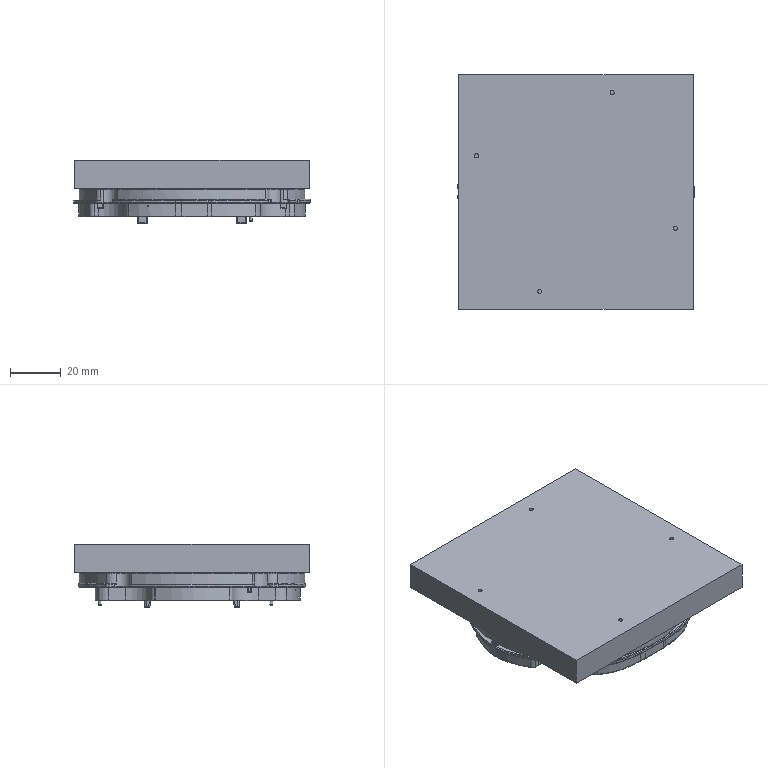NC program | NX | posted with a generic post | part box 92.935 x 92.1 x 24.829 mm
Lines 2470 to 3402 of 7643:
(PLANAR_MILL , TOOL : D3-9-D4-50-3T-ROUGH)
N4914 T15 M6
N4916 G53
N4918 G17 G0 G90 X17.469 Y27.537 S3500 M3
N4920 G43 Z21. H15
N4922 Z1.
N4924 G94 G1 Y26.515 Z0.991 F800.
N4926 X23.689 Z0.937
N4928 Y33.012 Z0.88
N4930 X17.801 Z0.829
N4932 X17.469 Z0.826
N4934 Y26.515 Z0.769
N4936 X23.689 Z0.715
N4938 Y33.012 Z0.658
N4940 X17.801 Z0.607
N4942 X17.469 Z0.604
N4944 Y26.515 Z0.547
N4946 X23.689 Z0.493
N4948 Y33.012 Z0.436
N4950 X17.801 Z0.385
N4952 X17.469 Z0.382
N4954 Y26.515 Z0.325
N4956 X23.689 Z0.271
N4958 Y33.012 Z0.214
N4960 X17.801 Z0.163
N4962 X17.469 Z0.16
N4964 Y26.515 Z0.103
N4966 X23.689 Z0.049
N4968 Y33.012 Z-0.008
N4970 X17.801 Z-0.059
N4972 X17.469 Z-0.062
N4974 Y26.515 Z-0.119
N4976 X23.689 Z-0.173
N4978 Y33.012 Z-0.23
N4980 X17.801 Z-0.281
N4982 X17.469 Z-0.284
N4984 Y26.515 Z-0.341
N4986 X23.689 Z-0.395
N4988 Y33.012 Z-0.452
N4990 X17.801 Z-0.503
N4992 X17.469 Z-0.506
N4994 Y26.515 Z-0.563
N4996 X23.689 Z-0.617
N4998 Y33.012 Z-0.674
N5000 X17.801 Z-0.725
N5002 X17.469 Z-0.728
N5004 Y26.515 Z-0.785
N5006 X23.689 Z-0.839
N5008 Y33.012 Z-0.896
N5010 X17.801 Z-0.947
N5012 X17.469 Z-0.95
N5014 Y26.515 Z-1.007
N5016 X23.689 Z-1.061
N5018 Y33.012 Z-1.118
N5020 X17.801 Z-1.169
N5022 X17.469 Z-1.172
N5024 Y26.515 Z-1.229
N5026 X23.689 Z-1.283
N5028 Y33.012 Z-1.34
N5030 X17.801 Z-1.391
N5032 X17.469 Z-1.394
N5034 Y26.515 Z-1.451
N5036 X23.689 Z-1.505
N5038 Y33.012 Z-1.562
N5040 X17.801 Z-1.613
N5042 X17.469 Z-1.616
N5044 Y26.515 Z-1.673
N5046 X23.689 Z-1.727
N5048 Y33.012 Z-1.784
N5050 X17.801 Z-1.835
N5052 X17.469 Z-1.838
N5054 Y26.515 Z-1.895
N5056 X23.689 Z-1.949
N5058 Y33.012 Z-2.006
N5060 X17.801 Z-2.057
N5062 X17.469 Z-2.06
N5064 Y26.515 Z-2.116
N5066 X23.689 Z-2.171
N5068 Y33.012 Z-2.227
N5070 X17.801 Z-2.279
N5072 X17.469 Z-2.282
N5074 Y26.515 Z-2.338
N5076 X23.689 Z-2.393
N5078 Y33.012 Z-2.449
N5080 X17.801 Z-2.501
N5082 X17.469 Z-2.504
N5084 Y26.515 Z-2.56
N5086 X23.689 Z-2.615
N5088 Y33.012 Z-2.671
N5090 X17.801 Z-2.723
N5092 X17.469 Z-2.726
N5094 Y26.515 Z-2.782
N5096 X23.689 Z-2.837
N5098 Y33.012 Z-2.893
N5100 X17.801 Z-2.945
N5102 X17.469 Z-2.948
N5104 Y26.515 Z-3.004
N5106 X23.689 Z-3.059
N5108 Y33.012 Z-3.115
N5110 X17.801 Z-3.167
N5112 X17.469 Z-3.17
N5114 Y26.515 Z-3.226
N5116 X23.689 Z-3.281
N5118 Y33.012 Z-3.337
N5120 X17.801 Z-3.389
N5122 X17.469 Z-3.392
N5124 Y26.515 Z-3.448
N5126 X23.689 Z-3.503
N5128 Y33.012 Z-3.559
N5130 X17.801 Z-3.611
N5132 X17.469 Z-3.614
N5134 Y26.515 Z-3.67
N5136 X23.689 Z-3.725
N5138 Y33.012 Z-3.781
N5140 X17.801 Z-3.833
N5142 X17.469 Z-3.836
N5144 Y26.515 Z-3.892
N5146 X23.689 Z-3.947
N5148 Y33.012 Z-4.003
N5150 X17.801 Z-4.055
N5152 X17.469 Z-4.058
N5154 Y26.515 Z-4.114
N5156 X23.689 Z-4.169
N5158 Y33.012 Z-4.225
N5160 X17.801 Z-4.277
N5162 X17.469 Z-4.279
N5164 Y26.515 Z-4.336
N5166 X23.689 Z-4.39
N5168 Y33.012 Z-4.447
N5170 X17.801 Z-4.499
N5172 X17.469 Z-4.501
N5174 Y26.515 Z-4.558
N5176 X23.689 Z-4.612
N5178 Y33.012 Z-4.669
N5180 X17.801 Z-4.721
N5182 X17.469 Z-4.723
N5184 Y26.515 Z-4.78
N5186 X23.689 Z-4.834
N5188 Y33.012 Z-4.891
N5190 X17.801 Z-4.942
N5192 X17.469 Z-4.945
N5194 Y26.515 Z-5.002
N5196 X23.689 Z-5.056
N5198 Y33.012 Z-5.113
N5200 X17.801 Z-5.164
N5202 X17.469 Z-5.167
N5204 Y26.515 Z-5.224
N5206 X23.689 Z-5.278
N5208 Y33.012 Z-5.335
N5210 X17.801 Z-5.386
N5212 X17.469 Z-5.389
N5214 Y26.515 Z-5.446
N5216 X23.689 Z-5.5
N5218 Y33.012 Z-5.557
N5220 X17.801 Z-5.608
N5222 X17.469 Z-5.611
N5224 Y26.515 Z-5.668
N5226 X23.689 Z-5.722
N5228 Y33.012 Z-5.779
N5230 X17.801 Z-5.83
N5232 X17.469 Z-5.833
N5234 Y26.515 Z-5.89
N5236 X23.689 Z-5.944
N5238 Y33.012 Z-6.001
N5240 X17.801 Z-6.052
N5242 X17.469 Z-6.055
N5244 Y26.515 Z-6.112
N5246 X23.689 Z-6.166
N5248 Y33.012 Z-6.223
N5250 X17.801 Z-6.274
N5252 X17.469 Z-6.277
N5254 Y26.515 Z-6.334
N5256 X23.689 Z-6.388
N5258 Y33.012 Z-6.445
N5260 X17.801 Z-6.496
N5262 X17.469 Z-6.499
N5264 Y26.515 Z-6.556
N5266 X23.689 Z-6.61
N5268 Y33.012 Z-6.667
N5270 X17.801 Z-6.718
N5272 X17.469 Z-6.721
N5274 Y26.515 Z-6.778
N5276 X23.689 Z-6.832
N5278 Y33.012 Z-6.889
N5280 X17.801 Z-6.94
N5282 X17.469 Z-6.943
N5284 Y26.515 Z-7.
N5286 X23.689 Z-7.054
N5288 Y33.012 Z-7.111
N5290 X17.801 Z-7.162
N5292 X17.469 Z-7.165
N5294 Y26.515 Z-7.222
N5296 X23.689 Z-7.276
N5298 Y33.012 Z-7.333
N5300 X17.801 Z-7.384
N5302 X17.469 Z-7.387
N5304 Y26.515 Z-7.444
N5306 X23.689 Z-7.498
N5308 Y33.012 Z-7.555
N5310 X17.801 Z-7.606
N5312 X17.469 Z-7.609
N5314 Y26.515 Z-7.666
N5316 X23.689 Z-7.72
N5318 Y33.012 Z-7.777
N5320 X17.801 Z-7.828
N5322 X17.469 Z-7.831
N5324 Y26.515 Z-7.888
N5326 X23.689 Z-7.942
N5328 Y33.012 Z-7.999
N5330 X17.801 Z-8.05
N5332 X17.469 Z-8.053
N5334 Y26.515 Z-8.11
N5336 X23.689 Z-8.164
N5338 Y33.012 Z-8.221
N5340 X17.801 Z-8.272
N5342 X17.469 Z-8.275
N5344 Y29.763 Z-8.303
N5346 Y26.515
N5348 X23.689
N5350 Y33.012
N5352 X17.801
N5354 X17.469
N5356 Y29.763
N5358 Z-7.303
N5360 G0 Z21.
N5362 X32.982 Y3.515
N5364 Z1.
N5366 G1 X37.639 Z0.959
N5368 X37.963 Y3.839 Z0.955
N5370 X37.928 Y10.192 Z0.9
N5372 X37.646 Y10.474 Z0.896
N5374 X37.558 Y10.509
N5376 X37.463 Z0.895
N5378 X32.293 Z0.85
N5380 X31.969 Y10.185 Z0.846
N5382 Y3.839 Z0.79
N5384 X32.293 Y3.515 Z0.786
N5386 X37.639 Z0.74
N5388 X37.963 Y3.839 Z0.736
N5390 X37.928 Y10.192 Z0.68
N5392 X37.646 Y10.474 Z0.677
N5394 X37.558 Y10.509 Z0.676
N5396 X37.463 Z0.675
N5398 X32.293 Z0.63
N5400 X31.969 Y10.185 Z0.626
N5402 Y3.839 Z0.57
N5404 X32.293 Y3.515 Z0.566
N5406 X37.639 Z0.52
N5408 X37.963 Y3.839 Z0.516
N5410 X37.928 Y10.192 Z0.46
N5412 X37.646 Y10.474 Z0.457
N5414 X37.558 Y10.509 Z0.456
N5416 X37.463 Z0.455
N5418 X32.293 Z0.41
N5420 X31.969 Y10.185 Z0.406
N5422 Y3.839 Z0.351
N5424 X32.293 Y3.515 Z0.347
N5426 X37.639 Z0.3
N5428 X37.963 Y3.839 Z0.296
N5430 X37.928 Y10.192 Z0.241
N5432 X37.646 Y10.474 Z0.237
N5434 X37.558 Y10.509 Z0.236
N5436 X37.463 Z0.235
N5438 X32.293 Z0.19
N5440 X31.969 Y10.185 Z0.186
N5442 Y3.839 Z0.131
N5444 X32.293 Y3.515 Z0.127
N5446 X37.639 Z0.08
N5448 X37.963 Y3.839 Z0.076
N5450 X37.928 Y10.192 Z0.021
N5452 X37.646 Y10.474 Z0.017
N5454 X37.558 Y10.509 Z0.016
N5456 X37.463
N5458 X32.293 Z-0.03
N5460 X31.969 Y10.185 Z-0.034
N5462 Y3.839 Z-0.089
N5464 X32.293 Y3.515 Z-0.093
N5466 X37.639 Z-0.14
N5468 X37.963 Y3.839 Z-0.144
N5470 X37.928 Y10.192 Z-0.199
N5472 X37.646 Y10.474 Z-0.203
N5474 X37.558 Y10.509
N5476 X37.463 Z-0.204
N5478 X32.293 Z-0.249
N5480 X31.969 Y10.185 Z-0.253
N5482 Y3.839 Z-0.309
N5484 X32.293 Y3.515 Z-0.313
N5486 X37.639 Z-0.359
N5488 X37.963 Y3.839 Z-0.363
N5490 X37.928 Y10.192 Z-0.419
N5492 X37.646 Y10.474 Z-0.422
N5494 X37.558 Y10.509 Z-0.423
N5496 X37.463 Z-0.424
N5498 X32.293 Z-0.469
N5500 X31.969 Y10.185 Z-0.473
N5502 Y3.839 Z-0.528
N5504 X32.293 Y3.515 Z-0.532
N5506 X37.639 Z-0.579
N5508 X37.963 Y3.839 Z-0.583
N5510 X37.928 Y10.192 Z-0.639
N5512 X37.646 Y10.474 Z-0.642
N5514 X37.558 Y10.509 Z-0.643
N5516 X37.463 Z-0.644
N5518 X32.293 Z-0.689
N5520 X31.969 Y10.185 Z-0.693
N5522 Y3.839 Z-0.748
N5524 X32.293 Y3.515 Z-0.752
N5526 X37.639 Z-0.799
N5528 X37.963 Y3.839 Z-0.803
N5530 X37.928 Y10.192 Z-0.858
N5532 X37.646 Y10.474 Z-0.862
N5534 X37.558 Y10.509 Z-0.863
N5536 X37.463 Z-0.864
N5538 X32.293 Z-0.909
N5540 X31.969 Y10.185 Z-0.913
N5542 Y3.839 Z-0.968
N5544 X32.293 Y3.515 Z-0.972
N5546 X37.639 Z-1.019
N5548 X37.963 Y3.839 Z-1.023
N5550 X37.928 Y10.192 Z-1.078
N5552 X37.646 Y10.474 Z-1.082
N5554 X37.558 Y10.509 Z-1.083
N5556 X37.463
N5558 X32.293 Z-1.128
N5560 X31.969 Y10.185 Z-1.132
N5562 Y3.839 Z-1.188
N5564 X32.293 Y3.515 Z-1.192
N5566 X37.639 Z-1.238
N5568 X37.963 Y3.839 Z-1.242
N5570 X37.928 Y10.192 Z-1.298
N5572 X37.646 Y10.474 Z-1.301
N5574 X37.558 Y10.509 Z-1.302
N5576 X37.463 Z-1.303
N5578 X32.293 Z-1.348
N5580 X31.969 Y10.185 Z-1.352
N5582 Y3.839 Z-1.408
N5584 X32.293 Y3.515 Z-1.412
N5586 X37.639 Z-1.458
N5588 X37.963 Y3.839 Z-1.462
N5590 X37.928 Y10.192 Z-1.518
N5592 X37.646 Y10.474 Z-1.521
N5594 X37.558 Y10.509 Z-1.522
N5596 X37.463 Z-1.523
N5598 X32.293 Z-1.568
N5600 X31.969 Y10.185 Z-1.572
N5602 Y3.839 Z-1.627
N5604 X32.293 Y3.515 Z-1.631
N5606 X37.639 Z-1.678
N5608 X37.963 Y3.839 Z-1.682
N5610 X37.928 Y10.192 Z-1.738
N5612 X37.646 Y10.474 Z-1.741
N5614 X37.558 Y10.509 Z-1.742
N5616 X37.463 Z-1.743
N5618 X32.293 Z-1.788
N5620 X31.969 Y10.185 Z-1.792
N5622 Y3.839 Z-1.847
N5624 X32.293 Y3.515 Z-1.851
N5626 X37.639 Z-1.898
N5628 X37.963 Y3.839 Z-1.902
N5630 X37.928 Y10.192 Z-1.957
N5632 X37.646 Y10.474 Z-1.961
N5634 X37.558 Y10.509 Z-1.962
N5636 X37.463
N5638 X32.293 Z-2.008
N5640 X31.969 Y10.185 Z-2.012
N5642 Y3.839 Z-2.067
N5644 X32.293 Y3.515 Z-2.071
N5646 X37.639 Z-2.118
N5648 X37.963 Y3.839 Z-2.122
N5650 X37.928 Y10.192 Z-2.177
N5652 X37.646 Y10.474 Z-2.181
N5654 X37.558 Y10.509
N5656 X37.463 Z-2.182
N5658 X32.293 Z-2.227
N5660 X31.969 Y10.185 Z-2.231
N5662 Y3.839 Z-2.287
N5664 X32.293 Y3.515 Z-2.291
N5666 X37.639 Z-2.337
N5668 X37.963 Y3.839 Z-2.341
N5670 X37.928 Y10.192 Z-2.397
N5672 X37.646 Y10.474 Z-2.4
N5674 X37.558 Y10.509 Z-2.401
N5676 X37.463 Z-2.402
N5678 X32.293 Z-2.447
N5680 X31.969 Y10.185 Z-2.451
N5682 Y3.839 Z-2.507
N5684 X32.293 Y3.515 Z-2.511
N5686 X37.639 Z-2.557
N5688 X37.963 Y3.839 Z-2.561
N5690 X37.928 Y10.192 Z-2.617
N5692 X37.646 Y10.474 Z-2.62
N5694 X37.558 Y10.509 Z-2.621
N5696 X37.463 Z-2.622
N5698 X32.293 Z-2.667
N5700 X31.969 Y10.185 Z-2.671
N5702 Y3.839 Z-2.726
N5704 X32.293 Y3.515 Z-2.73
N5706 X37.639 Z-2.777
N5708 X37.963 Y3.839 Z-2.781
N5710 X37.928 Y10.192 Z-2.836
N5712 X37.646 Y10.474 Z-2.84
N5714 X37.558 Y10.509 Z-2.841
N5716 X37.463 Z-2.842
N5718 X32.293 Z-2.887
N5720 X31.969 Y10.185 Z-2.891
N5722 Y3.839 Z-2.946
N5724 X32.293 Y3.515 Z-2.95
N5726 X37.639 Z-2.997
N5728 X37.963 Y3.839 Z-3.001
N5730 X37.928 Y10.192 Z-3.056
N5732 X37.646 Y10.474 Z-3.06
N5734 X37.558 Y10.509 Z-3.061
N5736 X37.463
N5738 X32.293 Z-3.107
N5740 X31.969 Y10.185 Z-3.111
N5742 Y3.839 Z-3.166
N5744 X32.293 Y3.515 Z-3.17
N5746 X37.639 Z-3.217
N5748 X37.963 Y3.839 Z-3.221
N5750 X37.928 Y10.192 Z-3.276
N5752 X37.646 Y10.474 Z-3.28
N5754 X37.558 Y10.509
N5756 X37.463 Z-3.281
N5758 X32.293 Z-3.326
N5760 X31.969 Y10.185 Z-3.33
N5762 Y3.839 Z-3.386
N5764 X32.293 Y3.515 Z-3.39
N5766 X37.639 Z-3.436
N5768 X37.963 Y3.839 Z-3.44
N5770 X37.928 Y10.192 Z-3.496
N5772 X37.646 Y10.474 Z-3.499
N5774 X37.558 Y10.509 Z-3.5
N5776 X37.463 Z-3.501
N5778 X32.293 Z-3.546
N5780 X31.969 Y10.185 Z-3.55
N5782 Y3.839 Z-3.605
N5784 X32.293 Y3.515 Z-3.609
N5786 X37.639 Z-3.656
N5788 X37.963 Y3.839 Z-3.66
N5790 X37.928 Y10.192 Z-3.716
N5792 X37.646 Y10.474 Z-3.719
N5794 X37.558 Y10.509 Z-3.72
N5796 X37.463 Z-3.721
N5798 X32.293 Z-3.766
N5800 X31.969 Y10.185 Z-3.77
N5802 Y3.839 Z-3.825
N5804 X32.293 Y3.515 Z-3.829
N5806 X37.639 Z-3.876
N5808 X37.963 Y3.839 Z-3.88
N5810 X37.928 Y10.192 Z-3.935
N5812 X37.646 Y10.474 Z-3.939
N5814 X37.558 Y10.509 Z-3.94
N5816 X37.463 Z-3.941
N5818 X32.293 Z-3.986
N5820 X31.969 Y10.185 Z-3.99
N5822 Y3.839 Z-4.045
N5824 X32.293 Y3.515 Z-4.049
N5826 X37.639 Z-4.096
N5828 X37.963 Y3.839 Z-4.1
N5830 X37.928 Y10.192 Z-4.155
N5832 X37.646 Y10.474 Z-4.159
N5834 X37.558 Y10.509
N5836 X37.463 Z-4.16
N5838 X32.293 Z-4.205
N5840 X31.969 Y10.185 Z-4.209
N5842 Y3.839 Z-4.265
N5844 X32.293 Y3.515 Z-4.269
N5846 X37.639 Z-4.315
N5848 X37.963 Y3.839 Z-4.319
N5850 X37.928 Y10.192 Z-4.375
N5852 X37.646 Y10.474 Z-4.378
N5854 X37.558 Y10.509 Z-4.379
N5856 X37.463 Z-4.38
N5858 X32.293 Z-4.425
N5860 X31.969 Y10.185 Z-4.429
N5862 Y3.839 Z-4.485
N5864 X32.293 Y3.515 Z-4.489
N5866 X37.639 Z-4.535
N5868 X37.963 Y3.839 Z-4.539
N5870 X37.928 Y10.192 Z-4.595
N5872 X37.646 Y10.474 Z-4.598
N5874 X37.558 Y10.509 Z-4.599
N5876 X37.463 Z-4.6
N5878 X32.293 Z-4.645
N5880 X31.969 Y10.185 Z-4.649
N5882 Y3.839 Z-4.704
N5884 X32.293 Y3.515 Z-4.708
N5886 X37.639 Z-4.755
N5888 X37.963 Y3.839 Z-4.759
N5890 X37.928 Y10.192 Z-4.815
N5892 X37.646 Y10.474 Z-4.818
N5894 X37.558 Y10.509 Z-4.819
N5896 X37.463 Z-4.82
N5898 X32.293 Z-4.865
N5900 X31.969 Y10.185 Z-4.869
N5902 Y3.839 Z-4.924
N5904 X32.293 Y3.515 Z-4.928
N5906 X37.639 Z-4.975
N5908 X37.963 Y3.839 Z-4.979
N5910 X37.928 Y10.192 Z-5.034
N5912 X37.646 Y10.474 Z-5.038
N5914 X37.558 Y10.509 Z-5.039
N5916 X37.463
N5918 X32.293 Z-5.085
N5920 X31.969 Y10.185 Z-5.089
N5922 Y3.839 Z-5.144
N5924 X32.293 Y3.515 Z-5.148
N5926 X37.639 Z-5.195
N5928 X37.963 Y3.839 Z-5.199
N5930 X37.928 Y10.192 Z-5.254
N5932 X37.646 Y10.474 Z-5.258
N5934 X37.558 Y10.509
N5936 X37.463 Z-5.259
N5938 X32.293 Z-5.304
N5940 X31.969 Y10.185 Z-5.308
N5942 Y3.839 Z-5.364
N5944 X32.293 Y3.515 Z-5.368
N5946 X37.639 Z-5.414
N5948 X37.963 Y3.839 Z-5.418
N5950 X37.928 Y10.192 Z-5.474
N5952 X37.646 Y10.474 Z-5.477
N5954 X37.558 Y10.509 Z-5.478
N5956 X37.463 Z-5.479
N5958 X32.293 Z-5.524
N5960 X31.969 Y10.185 Z-5.528
N5962 Y3.839 Z-5.584
N5964 X32.293 Y3.515 Z-5.588
N5966 X37.639 Z-5.634
N5968 X37.963 Y3.839 Z-5.638
N5970 X37.928 Y10.192 Z-5.694
N5972 X37.646 Y10.474 Z-5.697
N5974 X37.558 Y10.509 Z-5.698
N5976 X37.463 Z-5.699
N5978 X32.293 Z-5.744
N5980 X31.969 Y10.185 Z-5.748
N5982 Y3.839 Z-5.803
N5984 X32.293 Y3.515 Z-5.807
N5986 X37.639 Z-5.854
N5988 X37.963 Y3.839 Z-5.858
N5990 X37.928 Y10.192 Z-5.913
N5992 X37.646 Y10.474 Z-5.917
N5994 X37.558 Y10.509 Z-5.918
N5996 X37.463 Z-5.919
N5998 X32.293 Z-5.964
N6000 X31.969 Y10.185 Z-5.968
N6002 Y3.839 Z-6.023
N6004 X32.293 Y3.515 Z-6.027
N6006 X37.639 Z-6.074
N6008 X37.963 Y3.839 Z-6.078
N6010 X37.928 Y10.192 Z-6.133
N6012 X37.646 Y10.474 Z-6.137
N6014 X37.558 Y10.509 Z-6.138
N6016 X37.463
N6018 X32.293 Z-6.183
N6020 X31.969 Y10.185 Z-6.187
N6022 Y3.839 Z-6.243
N6024 X32.293 Y3.515 Z-6.247
N6026 X37.639 Z-6.294
N6028 X37.963 Y3.839 Z-6.298
N6030 X37.928 Y10.192 Z-6.353
N6032 X37.646 Y10.474 Z-6.357
N6034 X37.558 Y10.509
N6036 X37.463 Z-6.358
N6038 X32.293 Z-6.403
N6040 X31.969 Y10.185 Z-6.407
N6042 Y3.839 Z-6.463
N6044 X32.293 Y3.515 Z-6.467
N6046 X37.639 Z-6.513
N6048 X37.963 Y3.839 Z-6.517
N6050 X37.928 Y10.192 Z-6.573
N6052 X37.646 Y10.474 Z-6.576
N6054 X37.558 Y10.509 Z-6.577
N6056 X37.463 Z-6.578
N6058 X32.293 Z-6.623
N6060 X31.969 Y10.185 Z-6.627
N6062 Y3.839 Z-6.682
N6064 X32.293 Y3.515 Z-6.686
N6066 X37.639 Z-6.733
N6068 X37.963 Y3.839 Z-6.737
N6070 X37.928 Y10.192 Z-6.793
N6072 X37.646 Y10.474 Z-6.796
N6074 X37.558 Y10.509 Z-6.797
N6076 X37.463 Z-6.798
N6078 X32.293 Z-6.843
N6080 X31.969 Y10.185 Z-6.847
N6082 Y3.839 Z-6.902
N6084 X32.293 Y3.515 Z-6.906
N6086 X37.639 Z-6.953
N6088 X37.963 Y3.839 Z-6.957
N6090 X37.928 Y10.192 Z-7.012
N6092 X37.646 Y10.474 Z-7.016
N6094 X37.558 Y10.509 Z-7.017
N6096 X37.463 Z-7.018
N6098 X32.293 Z-7.063
N6100 X31.969 Y10.185 Z-7.067
N6102 Y3.839 Z-7.122
N6104 X32.293 Y3.515 Z-7.126
N6106 X37.639 Z-7.173
N6108 X37.963 Y3.839 Z-7.177
N6110 X37.928 Y10.192 Z-7.232
N6112 X37.646 Y10.474 Z-7.236
N6114 X37.558 Y10.509
N6116 X37.463 Z-7.237
N6118 X32.293 Z-7.282
N6120 X31.969 Y10.185 Z-7.286
N6122 Y3.839 Z-7.342
N6124 X32.293 Y3.515 Z-7.346
N6126 X37.639 Z-7.392
N6128 X37.963 Y3.839 Z-7.396
N6130 X37.928 Y10.192 Z-7.452
N6132 X37.646 Y10.474 Z-7.455
N6134 X37.558 Y10.509 Z-7.456
N6136 X37.463 Z-7.457
N6138 X32.293 Z-7.502
N6140 X31.969 Y10.185 Z-7.506
N6142 Y3.839 Z-7.562
N6144 X32.293 Y3.515 Z-7.566
N6146 X37.639 Z-7.612
N6148 X37.963 Y3.839 Z-7.616
N6150 X37.928 Y10.192 Z-7.672
N6152 X37.646 Y10.474 Z-7.675
N6154 X37.558 Y10.509 Z-7.676
N6156 X37.463 Z-7.677
N6158 X32.293 Z-7.722
N6160 X31.969 Y10.185 Z-7.726
N6162 Y3.839 Z-7.781
N6164 X32.293 Y3.515 Z-7.785
N6166 X37.639 Z-7.832
N6168 X37.963 Y3.839 Z-7.836
N6170 X37.928 Y10.192 Z-7.892
N6172 X37.646 Y10.474 Z-7.895
N6174 X37.558 Y10.509 Z-7.896
N6176 X37.463 Z-7.897
N6178 X32.293 Z-7.942
N6180 X31.969 Y10.185 Z-7.946
N6182 Y3.839 Z-8.001
N6184 X32.293 Y3.515 Z-8.005
N6186 X37.639 Z-8.052
N6188 X37.963 Y3.839 Z-8.056
N6190 X37.928 Y10.192 Z-8.111
N6192 X37.646 Y10.474 Z-8.115
N6194 X37.558 Y10.509 Z-8.116
N6196 X37.463
N6198 X32.293 Z-8.162
N6200 X31.969 Y10.185 Z-8.166
N6202 Y3.839 Z-8.221
N6204 X32.293 Y3.515 Z-8.225
N6206 X37.639 Z-8.272
N6208 X37.963 Y3.839 Z-8.276
N6210 Y7.012 Z-8.303
N6212 Y10.009
N6214 X37.984 Y10.108
N6216 X37.928 Y10.192
N6218 X37.646 Y10.474
N6220 X37.562 Y10.53
N6222 X37.463 Y10.509
N6224 X32.469
N6226 G3 X31.969 Y10.009 R0.5
N6228 G1 Y4.015
N6230 G3 X32.469 Y3.515 R0.5
N6232 G1 X37.463
N6234 G3 X37.963 Y4.015 R0.5
N6236 G1 Y7.012
N6238 Z-7.303
N6240 G0 Z21.
(PLANAR_MILL_4 , TOOL : D3-9-D4-50-3T-ROUGH)
N6242 X-36.227 Y19.536
N6244 Z1.
N6246 G1 X-36.188 Y19.49 Z0.997 F1200.
N6248 X-36.064 Y19.397 Z0.989
N6250 X-35.922 Y19.336 Z0.981
N6252 X-35.769 Y19.31 Z0.972
N6254 X-35.615 Y19.321 Z0.964
N6256 X-35.467 Y19.368 Z0.956
N6258 X-35.359 Y19.431 Z0.95
N6260 X-35.254 Y19.523 Z0.942
N6262 X-35.172 Y19.636 Z0.935
N6264 X-35.116 Y19.763 Z0.928
N6266 X-35.088 Y19.9 Z0.92
N6268 Y20.025 Z0.914
N6270 X-35.116 Y20.161 Z0.907
N6272 X-35.172 Y20.289 Z0.899
N6274 X-35.254 Y20.401 Z0.892
N6276 X-35.359 Y20.494 Z0.885
N6278 X-35.467 Y20.556 Z0.878
N6280 X-35.615 Y20.604 Z0.87
N6282 X-35.769 Y20.615 Z0.862
N6284 X-35.922 Y20.589 Z0.854
N6286 X-36.064 Y20.528 Z0.846
N6288 X-36.188 Y20.435 Z0.838
N6290 X-36.287 Y20.315 Z0.829
N6292 X-36.355 Y20.176 Z0.821
N6294 X-36.388 Y20.025 Z0.813
N6296 Y19.9 Z0.807
N6298 X-36.355 Y19.748 Z0.799
N6300 X-36.287 Y19.609 Z0.79
N6302 X-36.188 Y19.49 Z0.782
N6304 X-36.064 Y19.397 Z0.774
N6306 X-35.922 Y19.336 Z0.766
N6308 X-35.769 Y19.31 Z0.758
N6310 X-35.615 Y19.321 Z0.75
N6312 X-35.467 Y19.368 Z0.742
N6314 X-35.359 Y19.431 Z0.735
N6316 X-35.254 Y19.523 Z0.728
N6318 X-35.172 Y19.636 Z0.721
N6320 X-35.116 Y19.763 Z0.713
N6322 X-35.088 Y19.9 Z0.706
N6324 Y20.025 Z0.699
N6326 X-35.116 Y20.161 Z0.692
N6328 X-35.172 Y20.289 Z0.685
N6330 X-35.254 Y20.401 Z0.677
N6332 X-35.359 Y20.494 Z0.67
N6334 X-35.467 Y20.556 Z0.664
N6336 X-35.615 Y20.604 Z0.655
N6338 X-35.769 Y20.615 Z0.647
N6340 X-35.922 Y20.589 Z0.639
N6342 X-36.064 Y20.528 Z0.631
N6344 X-36.188 Y20.435 Z0.623
N6346 X-36.287 Y20.315 Z0.615
N6348 X-36.355 Y20.176 Z0.607
N6350 X-36.388 Y20.025 Z0.599
N6352 Y19.9 Z0.592
N6354 X-36.355 Y19.748 Z0.584
N6356 X-36.287 Y19.609 Z0.576
N6358 X-36.188 Y19.49 Z0.568
N6360 X-36.064 Y19.397 Z0.56
N6362 X-35.922 Y19.336 Z0.551
N6364 X-35.769 Y19.31 Z0.543
N6366 X-35.615 Y19.321 Z0.535
N6368 X-35.467 Y19.368 Z0.527
N6370 X-35.359 Y19.431 Z0.521
N6372 X-35.254 Y19.523 Z0.513
N6374 X-35.172 Y19.636 Z0.506
N6376 X-35.116 Y19.763 Z0.499
N6378 X-35.088 Y19.9 Z0.491
N6380 Y20.025 Z0.485
N6382 X-35.116 Y20.161 Z0.477
N6384 X-35.172 Y20.289 Z0.47
N6386 X-35.254 Y20.401 Z0.463
N6388 X-35.359 Y20.494 Z0.456
N6390 X-35.467 Y20.556 Z0.449
N6392 X-35.615 Y20.604 Z0.441
N6394 X-35.769 Y20.615 Z0.433
N6396 X-35.922 Y20.589 Z0.425
N6398 X-36.064 Y20.528 Z0.417
N6400 X-36.188 Y20.435 Z0.408
N6402 X-36.287 Y20.315 Z0.4
N6404 X-36.355 Y20.176 Z0.392
N6406 X-36.388 Y20.025 Z0.384
N6408 Y19.9 Z0.377
N6410 X-36.355 Y19.748 Z0.369
N6412 X-36.287 Y19.609 Z0.361
N6414 X-36.188 Y19.49 Z0.353
N6416 X-36.064 Y19.397 Z0.345
N6418 X-35.922 Y19.336 Z0.337
N6420 X-35.769 Y19.31 Z0.329
N6422 X-35.615 Y19.321 Z0.321
N6424 X-35.467 Y19.368 Z0.313
N6426 X-35.359 Y19.431 Z0.306
N6428 X-35.254 Y19.523 Z0.299
N6430 X-35.172 Y19.636 Z0.291
N6432 X-35.116 Y19.763 Z0.284
N6434 X-35.088 Y19.9 Z0.277
N6436 Y20.025 Z0.27
N6438 X-35.116 Y20.161 Z0.263
N6440 X-35.172 Y20.289 Z0.256
N6442 X-35.254 Y20.401 Z0.248
N6444 X-35.359 Y20.494 Z0.241
N6446 X-35.467 Y20.556 Z0.234
N6448 X-35.615 Y20.604 Z0.226
N6450 X-35.769 Y20.615 Z0.218
N6452 X-35.922 Y20.589 Z0.21
N6454 X-36.064 Y20.528 Z0.202
N6456 X-36.188 Y20.435 Z0.194
N6458 X-36.287 Y20.315 Z0.186
N6460 X-36.355 Y20.176 Z0.178
N6462 X-36.388 Y20.025 Z0.169
N6464 Y19.9 Z0.163
N6466 X-36.355 Y19.748 Z0.155
N6468 X-36.287 Y19.609 Z0.147
N6470 X-36.188 Y19.49 Z0.139
N6472 X-36.064 Y19.397 Z0.13
N6474 X-35.922 Y19.336 Z0.122
N6476 X-35.769 Y19.31 Z0.114
N6478 X-35.615 Y19.321 Z0.106
N6480 X-35.467 Y19.368 Z0.098
N6482 X-35.359 Y19.431 Z0.091
N6484 X-35.254 Y19.523 Z0.084
N6486 X-35.172 Y19.636 Z0.077
N6488 X-35.116 Y19.763 Z0.069
N6490 X-35.088 Y19.9 Z0.062
N6492 Y20.025 Z0.056
N6494 X-35.116 Y20.161 Z0.048
N6496 X-35.172 Y20.289 Z0.041
N6498 X-35.254 Y20.401 Z0.034
N6500 X-35.359 Y20.494 Z0.026
N6502 X-35.467 Y20.556 Z0.02
N6504 X-35.615 Y20.604 Z0.012
N6506 X-35.769 Y20.615 Z0.004
N6508 X-35.922 Y20.589 Z-0.004
N6510 X-36.064 Y20.528 Z-0.013
N6512 X-36.188 Y20.435 Z-0.021
N6514 X-36.287 Y20.315 Z-0.029
N6516 X-36.355 Y20.176 Z-0.037
N6518 X-36.388 Y20.025 Z-0.045
N6520 Y19.9 Z-0.052
N6522 X-36.355 Y19.748 Z-0.06
N6524 X-36.287 Y19.609 Z-0.068
N6526 X-36.188 Y19.49 Z-0.076
N6528 X-36.064 Y19.397 Z-0.084
N6530 X-35.922 Y19.336 Z-0.092
N6532 X-35.769 Y19.31 Z-0.1
N6534 X-35.615 Y19.321 Z-0.108
N6536 X-35.467 Y19.368 Z-0.117
N6538 X-35.359 Y19.431 Z-0.123
N6540 X-35.254 Y19.523 Z-0.13
N6542 X-35.172 Y19.636 Z-0.138
N6544 X-35.116 Y19.763 Z-0.145
N6546 X-35.088 Y19.9 Z-0.152
N6548 Y20.025 Z-0.159
N6550 X-35.116 Y20.161 Z-0.166
N6552 X-35.172 Y20.289 Z-0.174
N6554 X-35.254 Y20.401 Z-0.181
N6556 X-35.359 Y20.494 Z-0.188
N6558 X-35.467 Y20.556 Z-0.195
N6560 X-35.615 Y20.604 Z-0.203
N6562 X-35.769 Y20.615 Z-0.211
N6564 X-35.922 Y20.589 Z-0.219
N6566 X-36.064 Y20.528 Z-0.227
N6568 X-36.188 Y20.435 Z-0.235
N6570 X-36.287 Y20.315 Z-0.243
N6572 X-36.355 Y20.176 Z-0.252
N6574 X-36.388 Y20.025 Z-0.26
N6576 Y19.9 Z-0.266
N6578 X-36.355 Y19.748 Z-0.274
N6580 X-36.287 Y19.609 Z-0.282
N6582 X-36.188 Y19.49 Z-0.291
N6584 X-36.064 Y19.397 Z-0.299
N6586 X-35.922 Y19.336 Z-0.307
N6588 X-35.769 Y19.31 Z-0.315
N6590 X-35.615 Y19.321 Z-0.323
N6592 X-35.467 Y19.368 Z-0.331
N6594 X-35.359 Y19.431 Z-0.338
N6596 X-35.254 Y19.523 Z-0.345
N6598 X-35.172 Y19.636 Z-0.352
N6600 X-35.116 Y19.763 Z-0.36
N6602 X-35.088 Y19.9 Z-0.367
N6604 Y20.025 Z-0.373
N6606 X-35.116 Y20.161 Z-0.381
N6608 X-35.172 Y20.289 Z-0.388
N6610 X-35.254 Y20.401 Z-0.395
N6612 X-35.359 Y20.494 Z-0.403
N6614 X-35.467 Y20.556 Z-0.409
N6616 X-35.615 Y20.604 Z-0.417
N6618 X-35.769 Y20.615 Z-0.426
N6620 X-35.922 Y20.589 Z-0.434
N6622 X-36.064 Y20.528 Z-0.442
N6624 X-36.188 Y20.435 Z-0.45
N6626 X-36.287 Y20.315 Z-0.458
N6628 X-36.355 Y20.176 Z-0.466
N6630 X-36.388 Y20.025 Z-0.474
N6632 Y19.9 Z-0.481
N6634 X-36.355 Y19.748 Z-0.489
N6636 X-36.287 Y19.609 Z-0.497
N6638 X-36.188 Y19.49 Z-0.505
N6640 X-36.064 Y19.397 Z-0.513
N6642 X-35.922 Y19.336 Z-0.521
N6644 X-35.769 Y19.31 Z-0.529
N6646 X-35.615 Y19.321 Z-0.538
N6648 X-35.467 Y19.368 Z-0.546
N6650 X-35.359 Y19.431 Z-0.552
N6652 X-35.254 Y19.523 Z-0.56
N6654 X-35.172 Y19.636 Z-0.567
N6656 X-35.116 Y19.763 Z-0.574
N6658 X-35.088 Y19.9 Z-0.582
N6660 Y20.025 Z-0.588
N6662 X-35.116 Y20.161 Z-0.595
N6664 X-35.172 Y20.289 Z-0.603
N6666 X-35.254 Y20.401 Z-0.61
N6668 X-35.359 Y20.494 Z-0.617
N6670 X-35.467 Y20.556 Z-0.624
N6672 X-35.615 Y20.604 Z-0.632
N6674 X-35.769 Y20.615 Z-0.64
N6676 X-35.922 Y20.589 Z-0.648
N6678 X-36.064 Y20.528 Z-0.656
N6680 X-36.188 Y20.435 Z-0.664
N6682 X-36.287 Y20.315 Z-0.673
N6684 X-36.355 Y20.176 Z-0.681
N6686 X-36.388 Y20.025 Z-0.689
N6688 Y19.9 Z-0.695
N6690 X-36.355 Y19.748 Z-0.703
N6692 X-36.287 Y19.609 Z-0.712
N6694 X-36.188 Y19.49 Z-0.72
N6696 X-36.064 Y19.397 Z-0.728
N6698 X-35.922 Y19.336 Z-0.736
N6700 X-35.769 Y19.31 Z-0.744
N6702 X-35.615 Y19.321 Z-0.752
N6704 X-35.467 Y19.368 Z-0.76
N6706 X-35.359 Y19.431 Z-0.767
N6708 X-35.254 Y19.523 Z-0.774
N6710 X-35.172 Y19.636 Z-0.781
N6712 X-35.116 Y19.763 Z-0.789
N6714 X-35.088 Y19.9 Z-0.796
N6716 Y20.025 Z-0.803
N6718 X-35.116 Y20.161 Z-0.81
N6720 X-35.172 Y20.289 Z-0.817
N6722 X-35.254 Y20.401 Z-0.825
N6724 X-35.359 Y20.494 Z-0.832
N6726 X-35.467 Y20.556 Z-0.838
N6728 X-35.615 Y20.604 Z-0.847
N6730 X-35.769 Y20.615 Z-0.855
N6732 X-35.922 Y20.589 Z-0.863
N6734 X-36.064 Y20.528 Z-0.871
N6736 X-36.188 Y20.435 Z-0.879
N6738 X-36.287 Y20.315 Z-0.887
N6740 X-36.355 Y20.176 Z-0.895
N6742 X-36.388 Y20.025 Z-0.903
N6744 Y19.9 Z-0.91
N6746 X-36.355 Y19.748 Z-0.918
N6748 X-36.287 Y19.609 Z-0.926
N6750 X-36.188 Y19.49 Z-0.934
N6752 X-36.064 Y19.397 Z-0.942
N6754 X-35.922 Y19.336 Z-0.951
N6756 X-35.769 Y19.31 Z-0.959
N6758 X-35.615 Y19.321 Z-0.967
N6760 X-35.467 Y19.368 Z-0.975
N6762 X-35.359 Y19.431 Z-0.981
N6764 X-35.254 Y19.523 Z-0.989
N6766 X-35.172 Y19.636 Z-0.996